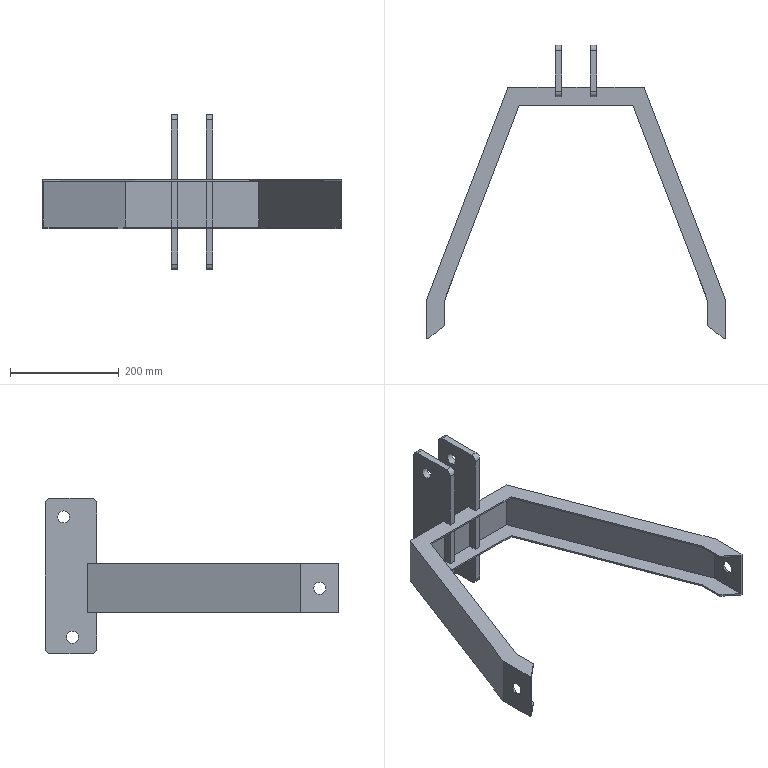Part | SolidWorks | features ICE 3, MirrorSolid 3, ExtruRefSurface 1, Thicken 1 | 1 solid | 74 faces | box 550 x 539.301 x 285 mm | volume 1145728 mm3 | plane 54 | cylinder 20 | commonest cylinder face diameters 22 x12 20 x8